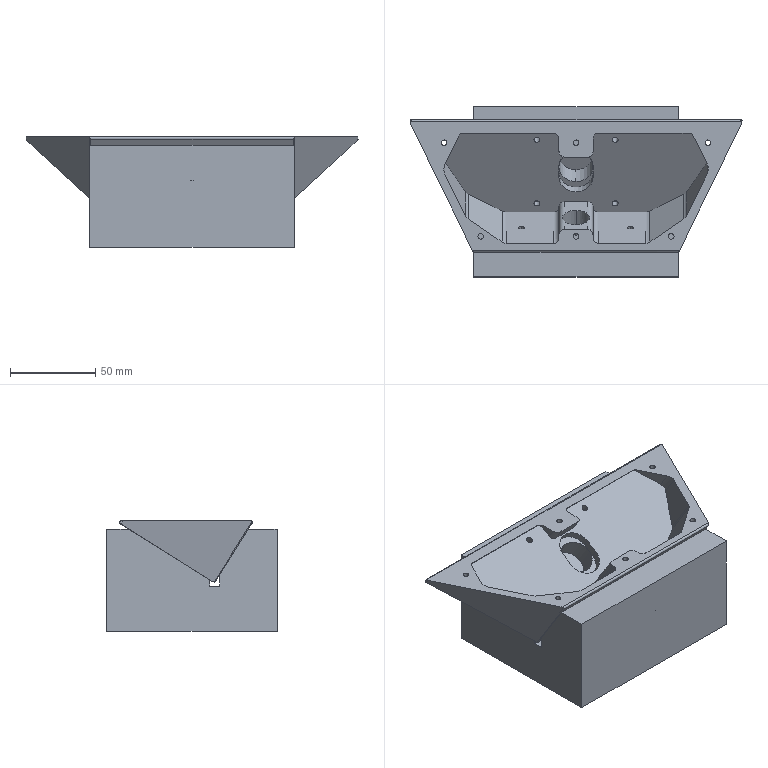NC program | Mastercam | posted with a generic post | part box 195.124 x 100 x 65 mm
Lines 8457 to 8876 of 16336:
N5280 T2 M6
N5290 G0 G90 G17 G57 X-102.94 Y-68.236 A180. S4000 M3
N5300 G43 H2 Z50.
N5310 Z-29.
N5320 G1 Z-31. F2000.
N5330 G41 D2 X-101.601 Y-67.361 F800.
N5340 G3 X-101.239 Y-66.691 I-.438 J.67
N5350 X-101.369 Y-66.254 I-.8 J0.
N5360 G2 X-109.974 Y-50.704 I101.369 J66.254
N5370 X-110.718 Y-47.313 I7.356 J3.391
N5380 X-109.893 Y-43.751 I8.1 J0.
N5390 G1 X-50.006 Y78.562
N5400 G2 X-42.731 Y83.1 I7.275 J-3.562
N5410 G1 X42.731
N5420 G2 X50.006 Y78.562 I0. J-8.1
N5430 G1 X109.893 Y-43.751
N5440 G2 X110.718 Y-47.313 I-7.275 J-3.562
N5450 X109.974 Y-50.704 I-8.1 J0.
N5460 X90.581 Y-80.376 I-109.974 J50.704
N5470 X84.522 Y-83.1 I-6.059 J5.376
N5480 G1 X-84.522
N5490 G2 X-90.581 Y-80.376 I0. J8.1
N5500 X-101.642 Y-65.834 I90.581 J80.376
N5510 G3 X-102.313 Y-65.469 I-.671 J-.435
N5520 X-102.748 Y-65.598 I0. J-.8
N5530 G1 G40 X-104.091 Y-66.468
N5540 X-102.94 Y-68.236
N5550 G41 D2 X-101.601 Y-67.361
N5560 G3 X-101.239 Y-66.691 I-.438 J.67
N5570 X-101.369 Y-66.254 I-.8 J0.
N5580 G2 X-109.974 Y-50.704 I101.369 J66.254
N5590 X-110.718 Y-47.313 I7.356 J3.391
N5600 X-109.893 Y-43.751 I8.1 J0.
N5610 G1 X-50.006 Y78.562
N5620 G2 X-42.731 Y83.1 I7.275 J-3.562
N5630 G1 X42.731
N5640 G2 X50.006 Y78.562 I0. J-8.1
N5650 G1 X109.893 Y-43.751
N5660 G2 X110.718 Y-47.313 I-7.275 J-3.562
N5670 X109.974 Y-50.704 I-8.1 J0.
N5680 X90.581 Y-80.376 I-109.974 J50.704
N5690 X84.522 Y-83.1 I-6.059 J5.376
N5700 G1 X-84.522
N5710 G2 X-90.581 Y-80.376 I0. J8.1
N5720 X-101.642 Y-65.834 I90.581 J80.376
N5730 G3 X-102.313 Y-65.469 I-.671 J-.435
N5740 X-102.748 Y-65.598 I0. J-.8
N5750 G1 G40 X-104.091 Y-66.468
N5760 G0 Z50.
N5770 M5
N5780 G91 G28 Z0.
N5790 A0.
N5800 M01
N5810 T3 M6
N5820 G0 G90 G17 G57 X0. Y-64. A180. S3000 M3
N5830 G43 H3 Z50.
N5840 G98 G81 Z-2. R1. F300.
N5850 X77.5 Y-25.269
N5860 X56. Y29.731
N5870 X0. Y64.
N5880 X-56. Y29.731
N5890 X-77.5 Y-25.269
N5900 G80
N5910 M5
N5920 G91 G0 G28 Z0.
N5930 A0.
N5940 M01
N5950 T14 M6
N5960 G0 G90 G17 G57 X77.5 Y-25.269 A180. S3000 M3
N5970 G43 H14 Z50.
N5980 G98 G83 Z-33. R1. Q3. F300.
N5990 X56. Y29.731
N6000 X-56.
N6010 X-77.5 Y-25.269
N6020 G80
N6030 M5
N6040 G91 G0 G28 Z0.
N6050 A0.
N6060 M01
N6070 T15 M6
N6080 G0 G90 G17 G57 X77.5 Y-25.269 A180. S2000 M3
N6090 G43 H15 Z50.
N6100 G98 G81 Z-10. R1. F100.
N6110 X56. Y29.731
N6120 X-56.
N6130 X-77.5 Y-25.269
N6140 G80
N6150 M5
N6160 G91 G0 G28 Z0.
N6170 A0.
N6180 M01
N6190 T16 M6
N6200 G0 G90 G17 G57 X0. Y-64. A180. S3000 M3
N6210 G43 H16 Z50.
N6220 G98 G83 Z-45. R1. Q4. F300.
N6230 Y64.
N6240 G80
N6250 M5
N6260 G91 G0 G28 Z0.
N6270 A0.
N6280 M01
N6290 T15 M6
N6300 G0 G90 G17 G57 X-49.3 Y-.4 A180. S4500 M3
N6310 G43 H15 Z50.
N6320 Z1.2
N6330 G1 Z.2 F2000.
N6340 G41 D15 X-48.5 F800.
N6350 G3 X-48.1 Y0. I0. J.4
N6360 X-50. Y1.9 Z.075 I-1.9 J0.
N6370 X-51.9 Y0. Z-.05 I0. J-1.9
N6380 X-50. Y-1.9 Z-.175 I1.9 J0.
N6390 X-48.1 Y0. Z-.3 I0. J1.9
N6400 X-50. Y1.9 Z-.425 I-1.9 J0.
N6410 X-51.9 Y0. Z-.55 I0. J-1.9
N6420 X-50. Y-1.9 Z-.675 I1.9 J0.
N6430 X-48.1 Y0. Z-.8 I0. J1.9
N6440 X-50. Y1.9 Z-.925 I-1.9 J0.
N6450 X-51.9 Y0. Z-1.05 I0. J-1.9
N6460 X-50. Y-1.9 Z-1.175 I1.9 J0.
N6470 X-48.1 Y0. Z-1.3 I0. J1.9
N6480 X-50. Y1.9 Z-1.425 I-1.9 J0.
N6490 X-51.9 Y0. Z-1.55 I0. J-1.9
N6500 X-50. Y-1.9 Z-1.675 I1.9 J0.
N6510 X-48.1 Y0. Z-1.8 I0. J1.9
N6520 X-50. Y1.9 Z-1.925 I-1.9 J0.
N6530 X-51.9 Y0. Z-2.05 I0. J-1.9
N6540 X-50. Y-1.9 Z-2.175 I1.9 J0.
N6550 X-48.1 Y0. Z-2.3 I0. J1.9
N6560 X-50. Y1.9 Z-2.425 I-1.9 J0.
N6570 X-51.9 Y0. Z-2.55 I0. J-1.9
N6580 X-50. Y-1.9 Z-2.675 I1.9 J0.
N6590 X-48.1 Y0. Z-2.8 I0. J1.9
N6600 X-50. Y1.9 Z-2.925 I-1.9 J0.
N6610 X-51.9 Y0. Z-3.05 I0. J-1.9
N6620 X-50. Y-1.9 Z-3.175 I1.9 J0.
N6630 X-48.1 Y0. Z-3.3 I0. J1.9
N6640 X-50. Y1.9 Z-3.425 I-1.9 J0.
N6650 X-51.9 Y0. Z-3.55 I0. J-1.9
N6660 X-50. Y-1.9 Z-3.675 I1.9 J0.
N6670 X-48.1 Y0. Z-3.8 I0. J1.9
N6680 X-50. Y1.9 Z-3.925 I-1.9 J0.
N6690 X-51.9 Y0. Z-4.05 I0. J-1.9
N6700 X-50. Y-1.9 Z-4.175 I1.9 J0.
N6710 X-48.1 Y0. Z-4.3 I0. J1.9
N6720 X-50. Y1.9 Z-4.425 I-1.9 J0.
N6730 X-51.537 Y1.117 Z-4.5 I0. J-1.9
N6740 X-51.9 Y0. I1.537 J-1.117
N6750 X-50. Y-1.9 I1.9 J0.
N6760 X-48.1 Y0. I0. J1.9
N6770 X-50. Y1.9 I-1.9 J0.
N6780 X-51.775 Y.678 I0. J-1.9
N6790 X-51.801 Y.536 I.374 J-.142
N6800 X-51.544 Y.162 I.4 J0.
N6810 G1 G40 X-50.797 Y-.124
N6820 G0 Z50.
N6830 X50.7 Y-.4
N6840 Z1.2
N6850 G1 Z.2 F2000.
N6860 G41 D15 X51.5 F800.
N6870 G3 X51.9 Y0. I0. J.4
N6880 X50. Y1.9 Z.075 I-1.9 J0.
N6890 X48.1 Y0. Z-.05 I0. J-1.9
N6900 X50. Y-1.9 Z-.175 I1.9 J0.
N6910 X51.9 Y0. Z-.3 I0. J1.9
N6920 X50. Y1.9 Z-.425 I-1.9 J0.
N6930 X48.1 Y0. Z-.55 I0. J-1.9
N6940 X50. Y-1.9 Z-.675 I1.9 J0.
N6950 X51.9 Y0. Z-.8 I0. J1.9
N6960 X50. Y1.9 Z-.925 I-1.9 J0.
N6970 X48.1 Y0. Z-1.05 I0. J-1.9
N6980 X50. Y-1.9 Z-1.175 I1.9 J0.
N6990 X51.9 Y0. Z-1.3 I0. J1.9
N7000 X50. Y1.9 Z-1.425 I-1.9 J0.
N7010 X48.1 Y0. Z-1.55 I0. J-1.9
N7020 X50. Y-1.9 Z-1.675 I1.9 J0.
N7030 X51.9 Y0. Z-1.8 I0. J1.9
N7040 X50. Y1.9 Z-1.925 I-1.9 J0.
N7050 X48.1 Y0. Z-2.05 I0. J-1.9
N7060 X50. Y-1.9 Z-2.175 I1.9 J0.
N7070 X51.9 Y0. Z-2.3 I0. J1.9
N7080 X50. Y1.9 Z-2.425 I-1.9 J0.
N7090 X48.1 Y0. Z-2.55 I0. J-1.9
N7100 X50. Y-1.9 Z-2.675 I1.9 J0.
N7110 X51.9 Y0. Z-2.8 I0. J1.9
N7120 X50. Y1.9 Z-2.925 I-1.9 J0.
N7130 X48.1 Y0. Z-3.05 I0. J-1.9
N7140 X50. Y-1.9 Z-3.175 I1.9 J0.
N7150 X51.9 Y0. Z-3.3 I0. J1.9
N7160 X50. Y1.9 Z-3.425 I-1.9 J0.
N7170 X48.1 Y0. Z-3.55 I0. J-1.9
N7180 X50. Y-1.9 Z-3.675 I1.9 J0.
N7190 X51.9 Y0. Z-3.8 I0. J1.9
N7200 X50. Y1.9 Z-3.925 I-1.9 J0.
N7210 X48.1 Y0. Z-4.05 I0. J-1.9
N7220 X50. Y-1.9 Z-4.175 I1.9 J0.
N7230 X51.9 Y0. Z-4.3 I0. J1.9
N7240 X50. Y1.9 Z-4.425 I-1.9 J0.
N7250 X48.463 Y1.117 Z-4.5 I0. J-1.9
N7260 X48.1 Y0. I1.537 J-1.117
N7270 X50. Y-1.9 I1.9 J0.
N7280 X51.9 Y0. I0. J1.9
N7290 X50. Y1.9 I-1.9 J0.
N7300 X48.225 Y.678 I0. J-1.9
N7310 X48.199 Y.536 I.374 J-.142
N7320 X48.456 Y.162 I.4 J0.
N7330 G1 G40 X49.203 Y-.124
N7340 G0 Z50.
N7350 M5
N7360 G91 G28 Z0.
N7370 A0.
N7380 M01
N7390 T17 M6
N7400 G0 G90 G17 G57 X-49.25 Y-.4 A180. S4500 M3
N7410 G43 H17 Z50.
N7420 Z1.2
N7430 G1 Z-4.5 F2000.
N7440 G41 D17 X-48.45 F400.
N7450 G3 X-48.05 Y0. I0. J.4
N7460 X-50. Y1.95 I-1.95 J0.
N7470 X-51.95 Y0. I0. J-1.95
N7480 X-50. Y-1.95 I1.95 J0.
N7490 X-48.05 Y0. I0. J1.95
N7500 X-48.114 Y.495 I-1.95 J0.
N7510 X-48.501 Y.793 I-.387 J-.102
N7520 X-48.602 Y.78 I0. J-.4
N7530 G1 G40 X-49.376 Y.577
N7540 X-49.25 Y-.4
N7550 G41 D17 X-48.45
N7560 G3 X-48.05 Y0. I0. J.4
N7570 X-50. Y1.95 I-1.95 J0.
N7580 X-51.95 Y0. I0. J-1.95
N7590 X-50. Y-1.95 I1.95 J0.
N7600 X-48.05 Y0. I0. J1.95
N7610 X-48.114 Y.495 I-1.95 J0.
N7620 X-48.501 Y.793 I-.387 J-.102
N7630 X-48.602 Y.78 I0. J-.4
N7640 G1 G40 X-49.376 Y.577
N7650 G0 Z50.
N7660 X50.75 Y-.4
N7670 Z1.2
N7680 G1 Z-4.5 F2000.
N7690 G41 D17 X51.55 F400.
N7700 G3 X51.95 Y0. I0. J.4
N7710 X50. Y1.95 I-1.95 J0.
N7720 X48.05 Y0. I0. J-1.95
N7730 X50. Y-1.95 I1.95 J0.
N7740 X51.95 Y0. I0. J1.95
N7750 X51.886 Y.495 I-1.95 J0.
N7760 X51.499 Y.793 I-.387 J-.102
N7770 X51.398 Y.78 I0. J-.4
N7780 G1 G40 X50.624 Y.577
N7790 X50.75 Y-.4
N7800 G41 D17 X51.55
N7810 G3 X51.95 Y0. I0. J.4
N7820 X50. Y1.95 I-1.95 J0.
N7830 X48.05 Y0. I0. J-1.95
N7840 X50. Y-1.95 I1.95 J0.
N7850 X51.95 Y0. I0. J1.95
N7860 X51.886 Y.495 I-1.95 J0.
N7870 X51.499 Y.793 I-.387 J-.102
N7880 X51.398 Y.78 I0. J-.4
N7890 G1 G40 X50.624 Y.577
N7900 G0 Z50.
N7910 M5
N7920 G91 G28 Z0.
N7930 A0.
N7940 M01
N7950 T3 M6
N7960 G0 G90 G17 G57 X58.1 Y29.431 A180. S4000 M3
N7970 G43 H3 Z50.
N7980 Z1.
N7990 G1 Z-1.3 F2000.
N8000 G41 D3 X58.7 F600.
N8010 G3 X59. Y29.731 I0. J.3
N8020 X56. Y32.731 I-3. J0.
N8030 X53. Y29.731 I0. J-3.
N8040 X56. Y26.731 I3. J0.
N8050 X59. Y29.731 I0. J3.
N8060 X58.958 Y30.228 I-3. J0.
N8070 X58.663 Y30.477 I-.295 J-.05
N8080 X58.613 Y30.474 I0. J-.299
N8090 G1 G40 X58.021 Y30.375
N8100 G0 Z50.
N8110 X79.6 Y-25.569
N8120 Z1.
N8130 G1 Z-1.3 F2000.
N8140 G41 D3 X80.2 F600.
N8150 G3 X80.5 Y-25.269 I0. J.3
N8160 X77.5 Y-22.269 I-3. J0.
N8170 X74.5 Y-25.269 I0. J-3.
N8180 X77.5 Y-28.269 I3. J0.
N8190 X80.5 Y-25.269 I0. J3.
N8200 X80.458 Y-24.772 I-3. J0.
N8210 X80.163 Y-24.523 I-.295 J-.05
N8220 X80.113 Y-24.526 I0. J-.299
N8230 G1 G40 X79.521 Y-24.625
N8240 G0 Z50.
N8250 X-75.4 Y-25.569
N8260 Z1.
N8270 G1 Z-1.3 F2000.
N8280 G41 D3 X-74.8 F600.
N8290 G3 X-74.5 Y-25.269 I0. J.3
N8300 X-77.5 Y-22.269 I-3. J0.
N8310 X-80.5 Y-25.269 I0. J-3.
N8320 X-77.5 Y-28.269 I3. J0.
N8330 X-74.5 Y-25.269 I0. J3.
N8340 X-74.542 Y-24.772 I-3. J0.
N8350 X-74.837 Y-24.523 I-.295 J-.05
N8360 X-74.887 Y-24.526 I0. J-.299
N8370 G1 G40 X-75.479 Y-24.625
N8380 G0 Z50.
N8390 X-53.9 Y29.431
N8400 Z1.
N8410 G1 Z-1.3 F2000.
N8420 G41 D3 X-53.3 F600.
N8430 G3 X-53. Y29.731 I0. J.3
N8440 X-56. Y32.731 I-3. J0.
N8450 X-59. Y29.731 I0. J-3.
N8460 X-56. Y26.731 I3. J0.
N8470 X-53. Y29.731 I0. J3.
N8480 X-53.042 Y30.228 I-3. J0.
N8490 X-53.337 Y30.477 I-.295 J-.05
N8500 X-53.387 Y30.474 I0. J-.299
N8510 G1 G40 X-53.979 Y30.375
N8520 G0 Z50.
N8530 X-104.457 Y-46.747
N8540 Z1.
N8550 G1 Z-1.3 F2000.
N8560 G41 D3 X-103.918 Y-47.011 F600.
N8570 G3 X-103.786 Y-47.042 I.132 J.27
N8580 X-103.516 Y-46.873 I0. J.301
N8590 G1 X-43.629 Y75.44
N8600 G2 X-42.731 Y76. I.898 J-.44
N8610 G1 X42.731
N8620 G2 X43.629 Y75.44 I0. J-1.
N8630 G1 X103.516 Y-46.873
N8640 G2 X103.618 Y-47.313 I-.898 J-.44
N8650 X103.526 Y-47.731 I-1. J0.
N8660 X85.27 Y-75.664 I-103.526 J47.731
N8670 X84.522 Y-76. I-.748 J.664
N8680 G1 X-84.522
N8690 G2 X-85.27 Y-75.664 I0. J1.
N8700 X-103.526 Y-47.731 I85.27 J75.664
N8710 X-103.618 Y-47.313 I.908 J.418
N8720 X-103.516 Y-46.873 I1. J0.
N8730 G1 X-103.296 Y-46.424
N8740 G3 X-103.265 Y-46.292 I-.27 J.132
N8750 X-103.434 Y-46.023 I-.301 J0.
N8760 G1 G40 X-103.973 Y-45.759
N8770 G0 Z50.
N8780 X-45.9 Y-.3
N8790 Z1.
N8800 G1 Z-1.3 F2000.
N8810 G41 D3 X-45.3 F600.
N8820 G3 X-45. Y0. I0. J.3
N8830 X-50. Y5. I-5. J0.
N8840 X-55. Y0. I0. J-5.
N8850 X-50. Y-5. I5. J0.
N8860 X-45. Y0. I0. J5.
N8870 X-45.025 Y.499 I-5. J0.
N8880 X-45.323 Y.769 I-.298 J-.03
N8890 X-45.353 Y.768 I0. J-.3
N8900 G1 G40 X-45.95 Y.708
N8910 G0 Z50.
N8920 X54.1 Y-.3
N8930 Z1.
N8940 G1 Z-1.3 F2000.
N8950 G41 D3 X54.7 F600.
N8960 G3 X55. Y0. I0. J.3
N8970 X50. Y5. I-5. J0.
N8980 X45. Y0. I0. J-5.
N8990 X50. Y-5. I5. J0.
N9000 X55. Y0. I0. J5.
N9010 X54.975 Y.499 I-5. J0.
N9020 X54.677 Y.769 I-.298 J-.03
N9030 X54.647 Y.768 I0. J-.3
N9040 G1 G40 X54.05 Y.708
N9050 G0 Z50.
N9060 X2.6 Y63.7
N9070 Z1.
N9080 G1 Z-1.3 F2000.
N9090 G41 D3 X3.2 F600.
N9100 G3 X3.5 Y64. I0. J.3
N9110 X0. Y67.5 I-3.5 J0.
N9120 X-3.5 Y64. I0. J-3.5
N9130 X0. Y60.5 I3.5 J0.
N9140 X3.5 Y64. I0. J3.5
N9150 X3.464 Y64.498 I-3.5 J0.
N9160 X3.167 Y64.756 I-.297 J-.042
N9170 X3.125 Y64.753 I0. J-.3
N9180 G1 G40 X2.531 Y64.667
N9190 G0 Z50.
N9200 X2.6 Y-64.3
N9210 Z1.
N9220 G1 Z-1.3 F2000.
N9230 G41 D3 X3.2 F600.
N9240 G3 X3.5 Y-64. I0. J.3
N9250 X0. Y-60.5 I-3.5 J0.
N9260 X-3.5 Y-64. I0. J-3.5
N9270 X0. Y-67.5 I3.5 J0.
N9280 X3.5 Y-64. I0. J3.5
N9290 X3.464 Y-63.502 I-3.5 J0.
N9300 X3.167 Y-63.244 I-.297 J-.042
N9310 X3.125 Y-63.247 I0. J-.3
N9320 G1 G40 X2.531 Y-63.333
N9330 G0 Z50.
N9340 M5
N9350 G91 G28 Z0.
N9360 A0.
N9370 M01
N9380 T18 M6
N9390 G0 G90 G17 G58 X0. Y-64. A0. S1000 M3
N9400 G43 H18 Z50.
N9410 G98 G81 Z-20. R6. F100.
N9420 Y64.
N9430 G80
N9440 M5
N9450 G91 G0 G28 Z0.
N9460 A0.
N9470 M01